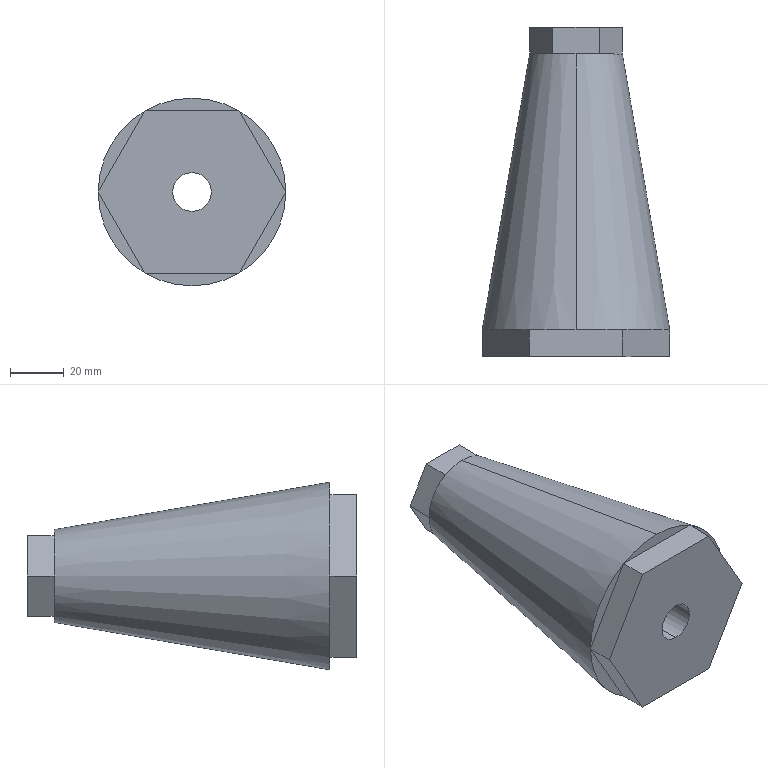Part | SolidWorks | features Extrusion 1, HoleWzd 1, ICE 1, Revolution 1 | 1 solid | 30 faces | box 70 x 123 x 70 mm | volume 249186 mm3 | plane 26 | cylinder 2 | cone 2 | commonest cylinder face diameters 14.5 x2
STEP:
#1=CARTESIAN_POINT('',(0.,-113.,-7.25));
#2=VERTEX_POINT('',#1);
#3=CARTESIAN_POINT('',(0.,-113.,7.25));
#4=VERTEX_POINT('',#3);
#5=CARTESIAN_POINT('',(0.,-113.,0.));
#6=DIRECTION('',(0.,1.,0.));
#7=DIRECTION('',(0.,0.,1.));
#8=AXIS2_PLACEMENT_3D('',#5,#6,#7);
#9=CIRCLE('',#8,7.25);
#10=EDGE_CURVE('',#2,#4,#9,.T.);
#11=ORIENTED_EDGE('',*,*,#10,.F.);
#12=CARTESIAN_POINT('',(0.,10.,-7.25));
#13=VERTEX_POINT('',#12);
#14=CARTESIAN_POINT('',(0.,10.,-7.25));
#15=DIRECTION('',(0.,1.,0.));
#16=VECTOR('',#15,1000.);
#17=LINE('',#14,#16);
#18=EDGE_CURVE('',#2,#13,#17,.T.);
#19=ORIENTED_EDGE('',*,*,#18,.T.);
#20=CARTESIAN_POINT('',(0.,10.,7.25));
#21=VERTEX_POINT('',#20);
#22=CARTESIAN_POINT('',(0.,10.,0.));
#23=DIRECTION('',(0.,1.,0.));
#24=DIRECTION('',(0.,0.,1.));
#25=AXIS2_PLACEMENT_3D('',#22,#23,#24);
#26=CIRCLE('',#25,7.25);
#27=EDGE_CURVE('',#13,#21,#26,.T.);
#28=ORIENTED_EDGE('',*,*,#27,.T.);
#29=CARTESIAN_POINT('',(0.,10.,7.25));
#30=DIRECTION('',(0.,1.,0.));
#31=VECTOR('',#30,1000.);
#32=LINE('',#29,#31);
#33=EDGE_CURVE('',#4,#21,#32,.T.);
#34=ORIENTED_EDGE('',*,*,#33,.F.);
#35=EDGE_LOOP('',(#11,#19,#28,#34));
#36=FACE_OUTER_BOUND('',#35,.T.);
#37=CARTESIAN_POINT('',(0.,10.,0.));
#38=DIRECTION('',(0.,1.,0.));
#39=DIRECTION('',(0.,0.,1.));
#40=AXIS2_PLACEMENT_3D('',#37,#38,#39);
#41=CYLINDRICAL_SURFACE('',#40,7.25);
#42=ADVANCED_FACE('',(#36),#41,.F.);
#43=CARTESIAN_POINT('',(8.66,0.,15.));
#44=VERTEX_POINT('',#43);
#45=CARTESIAN_POINT('',(0.,0.,17.321));
#46=VERTEX_POINT('',#45);
#47=CARTESIAN_POINT('',(0.,0.,0.));
#48=DIRECTION('',(0.,-1.,0.));
#49=DIRECTION('',(0.,0.,-1.));
#50=AXIS2_PLACEMENT_3D('',#47,#48,#49);
#51=CIRCLE('',#50,17.321);
#52=EDGE_CURVE('',#44,#46,#51,.T.);
#53=ORIENTED_EDGE('',*,*,#52,.T.);
#54=CARTESIAN_POINT('',(0.,-103.,35.));
#55=VERTEX_POINT('',#54);
#56=CARTESIAN_POINT('',(0.,-103.,35.));
#57=DIRECTION('',(0.,-0.9856,0.1692));
#58=VECTOR('',#57,1000.);
#59=LINE('',#56,#58);
#60=EDGE_CURVE('',#46,#55,#59,.T.);
#61=ORIENTED_EDGE('',*,*,#60,.T.);
#62=CARTESIAN_POINT('',(17.5,-103.,30.311));
#63=VERTEX_POINT('',#62);
#64=CARTESIAN_POINT('',(0.,-103.,0.));
#65=DIRECTION('',(0.,-1.,0.));
#66=DIRECTION('',(0.,0.,-1.));
#67=AXIS2_PLACEMENT_3D('',#64,#65,#66);
#68=CIRCLE('',#67,35.);
#69=EDGE_CURVE('',#63,#55,#68,.T.);
#70=ORIENTED_EDGE('',*,*,#69,.F.);
#71=CARTESIAN_POINT('',(35.,-103.,0.));
#72=VERTEX_POINT('',#71);
#73=CARTESIAN_POINT('',(0.,-103.,0.));
#74=DIRECTION('',(0.,-1.,0.));
#75=DIRECTION('',(0.,0.,-1.));
#76=AXIS2_PLACEMENT_3D('',#73,#74,#75);
#77=CIRCLE('',#76,35.);
#78=EDGE_CURVE('',#72,#63,#77,.T.);
#79=ORIENTED_EDGE('',*,*,#78,.F.);
#80=CARTESIAN_POINT('',(17.5,-103.,-30.311));
#81=VERTEX_POINT('',#80);
#82=CARTESIAN_POINT('',(0.,-103.,0.));
#83=DIRECTION('',(0.,-1.,0.));
#84=DIRECTION('',(0.,0.,-1.));
#85=AXIS2_PLACEMENT_3D('',#82,#83,#84);
#86=CIRCLE('',#85,35.);
#87=EDGE_CURVE('',#81,#72,#86,.T.);
#88=ORIENTED_EDGE('',*,*,#87,.F.);
#89=CARTESIAN_POINT('',(0.,-103.,-35.));
#90=VERTEX_POINT('',#89);
#91=CARTESIAN_POINT('',(0.,-103.,0.));
#92=DIRECTION('',(0.,-1.,0.));
#93=DIRECTION('',(0.,0.,-1.));
#94=AXIS2_PLACEMENT_3D('',#91,#92,#93);
#95=CIRCLE('',#94,35.);
#96=EDGE_CURVE('',#90,#81,#95,.T.);
#97=ORIENTED_EDGE('',*,*,#96,.F.);
#98=CARTESIAN_POINT('',(0.,0.,-17.321));
#99=VERTEX_POINT('',#98);
#100=CARTESIAN_POINT('',(0.,-103.,-35.));
#101=DIRECTION('',(0.,-0.9856,-0.1692));
#102=VECTOR('',#101,1000.);
#103=LINE('',#100,#102);
#104=EDGE_CURVE('',#99,#90,#103,.T.);
#105=ORIENTED_EDGE('',*,*,#104,.F.);
#106=CARTESIAN_POINT('',(8.66,0.,-15.));
#107=VERTEX_POINT('',#106);
#108=CARTESIAN_POINT('',(0.,0.,0.));
#109=DIRECTION('',(0.,-1.,0.));
#110=DIRECTION('',(0.,0.,-1.));
#111=AXIS2_PLACEMENT_3D('',#108,#109,#110);
#112=CIRCLE('',#111,17.321);
#113=EDGE_CURVE('',#99,#107,#112,.T.);
#114=ORIENTED_EDGE('',*,*,#113,.T.);
#115=CARTESIAN_POINT('',(17.321,0.,0.));
#116=VERTEX_POINT('',#115);
#117=CARTESIAN_POINT('',(0.,0.,0.));
#118=DIRECTION('',(0.,-1.,0.));
#119=DIRECTION('',(0.,0.,-1.));
#120=AXIS2_PLACEMENT_3D('',#117,#118,#119);
#121=CIRCLE('',#120,17.321);
#122=EDGE_CURVE('',#107,#116,#121,.T.);
#123=ORIENTED_EDGE('',*,*,#122,.T.);
#124=CARTESIAN_POINT('',(0.,0.,0.));
#125=DIRECTION('',(0.,-1.,0.));
#126=DIRECTION('',(0.,0.,-1.));
#127=AXIS2_PLACEMENT_3D('',#124,#125,#126);
#128=CIRCLE('',#127,17.321);
#129=EDGE_CURVE('',#116,#44,#128,.T.);
#130=ORIENTED_EDGE('',*,*,#129,.T.);
#131=EDGE_LOOP('',(#53,#61,#70,#79,#88,#97,#105,#114,#123,#130));
#132=FACE_OUTER_BOUND('',#131,.T.);
#133=CARTESIAN_POINT('',(0.,-103.,0.));
#134=DIRECTION('',(0.,-1.,0.));
#135=DIRECTION('',(0.,0.,-1.));
#136=AXIS2_PLACEMENT_3D('',#133,#134,#135);
#137=CONICAL_SURFACE('',#136,35.,0.17);
#138=ADVANCED_FACE('',(#132),#137,.T.);
#139=CARTESIAN_POINT('',(35.,-103.,0.));
#140=DIRECTION('',(-0.5,0.,0.866));
#141=VECTOR('',#140,1000.);
#142=LINE('',#139,#141);
#143=EDGE_CURVE('',#72,#63,#142,.T.);
#144=ORIENTED_EDGE('',*,*,#143,.F.);
#145=ORIENTED_EDGE('',*,*,#78,.T.);
#146=EDGE_LOOP('',(#144,#145));
#147=FACE_OUTER_BOUND('',#146,.T.);
#148=CARTESIAN_POINT('',(35.,-103.,0.));
#149=DIRECTION('',(0.,-1.,0.));
#150=DIRECTION('',(0.,0.,-1.));
#151=AXIS2_PLACEMENT_3D('',#148,#149,#150);
#152=PLANE('',#151);
#153=ADVANCED_FACE('',(#147),#152,.T.);
#154=CARTESIAN_POINT('',(17.5,-103.,-30.311));
#155=DIRECTION('',(0.5,0.,0.866));
#156=VECTOR('',#155,1000.);
#157=LINE('',#154,#156);
#158=EDGE_CURVE('',#81,#72,#157,.T.);
#159=ORIENTED_EDGE('',*,*,#158,.F.);
#160=ORIENTED_EDGE('',*,*,#87,.T.);
#161=EDGE_LOOP('',(#159,#160));
#162=FACE_OUTER_BOUND('',#161,.T.);
#163=CARTESIAN_POINT('',(35.,-103.,0.));
#164=DIRECTION('',(0.,-1.,0.));
#165=DIRECTION('',(0.,0.,-1.));
#166=AXIS2_PLACEMENT_3D('',#163,#164,#165);
#167=PLANE('',#166);
#168=ADVANCED_FACE('',(#162),#167,.T.);
#169=CARTESIAN_POINT('',(-17.5,-103.,-30.311));
#170=VERTEX_POINT('',#169);
#171=CARTESIAN_POINT('',(-17.5,-103.,-30.311));
#172=DIRECTION('',(1.,0.,0.));
#173=VECTOR('',#172,1000.);
#174=LINE('',#171,#173);
#175=EDGE_CURVE('',#170,#81,#174,.T.);
#176=ORIENTED_EDGE('',*,*,#175,.F.);
#177=CARTESIAN_POINT('',(0.,-103.,0.));
#178=DIRECTION('',(0.,-1.,0.));
#179=DIRECTION('',(0.,0.,-1.));
#180=AXIS2_PLACEMENT_3D('',#177,#178,#179);
#181=CIRCLE('',#180,35.);
#182=EDGE_CURVE('',#170,#90,#181,.T.);
#183=ORIENTED_EDGE('',*,*,#182,.T.);
#184=ORIENTED_EDGE('',*,*,#96,.T.);
#185=EDGE_LOOP('',(#176,#183,#184));
#186=FACE_OUTER_BOUND('',#185,.T.);
#187=CARTESIAN_POINT('',(35.,-103.,0.));
#188=DIRECTION('',(0.,-1.,0.));
#189=DIRECTION('',(0.,0.,-1.));
#190=AXIS2_PLACEMENT_3D('',#187,#188,#189);
#191=PLANE('',#190);
#192=ADVANCED_FACE('',(#186),#191,.T.);
#193=CARTESIAN_POINT('',(-35.,-103.,0.));
#194=VERTEX_POINT('',#193);
#195=CARTESIAN_POINT('',(-35.,-103.,0.));
#196=DIRECTION('',(0.5,0.,-0.866));
#197=VECTOR('',#196,1000.);
#198=LINE('',#195,#197);
#199=EDGE_CURVE('',#194,#170,#198,.T.);
#200=ORIENTED_EDGE('',*,*,#199,.F.);
#201=CARTESIAN_POINT('',(0.,-103.,0.));
#202=DIRECTION('',(0.,-1.,0.));
#203=DIRECTION('',(0.,0.,-1.));
#204=AXIS2_PLACEMENT_3D('',#201,#202,#203);
#205=CIRCLE('',#204,35.);
#206=EDGE_CURVE('',#194,#170,#205,.T.);
#207=ORIENTED_EDGE('',*,*,#206,.T.);
#208=EDGE_LOOP('',(#200,#207));
#209=FACE_OUTER_BOUND('',#208,.T.);
#210=CARTESIAN_POINT('',(35.,-103.,0.));
#211=DIRECTION('',(0.,-1.,0.));
#212=DIRECTION('',(0.,0.,-1.));
#213=AXIS2_PLACEMENT_3D('',#210,#211,#212);
#214=PLANE('',#213);
#215=ADVANCED_FACE('',(#209),#214,.T.);
#216=CARTESIAN_POINT('',(-17.5,-103.,30.311));
#217=VERTEX_POINT('',#216);
#218=CARTESIAN_POINT('',(-17.5,-103.,30.311));
#219=DIRECTION('',(-0.5,0.,-0.866));
#220=VECTOR('',#219,1000.);
#221=LINE('',#218,#220);
#222=EDGE_CURVE('',#217,#194,#221,.T.);
#223=ORIENTED_EDGE('',*,*,#222,.F.);
#224=CARTESIAN_POINT('',(0.,-103.,0.));
#225=DIRECTION('',(0.,-1.,0.));
#226=DIRECTION('',(0.,0.,-1.));
#227=AXIS2_PLACEMENT_3D('',#224,#225,#226);
#228=CIRCLE('',#227,35.);
#229=EDGE_CURVE('',#217,#194,#228,.T.);
#230=ORIENTED_EDGE('',*,*,#229,.T.);
#231=EDGE_LOOP('',(#223,#230));
#232=FACE_OUTER_BOUND('',#231,.T.);
#233=CARTESIAN_POINT('',(35.,-103.,0.));
#234=DIRECTION('',(0.,-1.,0.));
#235=DIRECTION('',(0.,0.,-1.));
#236=AXIS2_PLACEMENT_3D('',#233,#234,#235);
#237=PLANE('',#236);
#238=ADVANCED_FACE('',(#232),#237,.T.);
#239=CARTESIAN_POINT('',(-8.66,0.,15.));
#240=VERTEX_POINT('',#239);
#241=CARTESIAN_POINT('',(-8.66,0.,15.));
#242=DIRECTION('',(1.,0.,0.));
#243=VECTOR('',#242,1000.);
#244=LINE('',#241,#243);
#245=EDGE_CURVE('',#240,#44,#244,.T.);
#246=ORIENTED_EDGE('',*,*,#245,.T.);
#247=CARTESIAN_POINT('',(8.66,10.,15.));
#248=VERTEX_POINT('',#247);
#249=CARTESIAN_POINT('',(8.66,10.,15.));
#250=DIRECTION('',(0.,-1.,0.));
#251=VECTOR('',#250,1000.);
#252=LINE('',#249,#251);
#253=EDGE_CURVE('',#248,#44,#252,.T.);
#254=ORIENTED_EDGE('',*,*,#253,.F.);
#255=CARTESIAN_POINT('',(-8.66,10.,15.));
#256=VERTEX_POINT('',#255);
#257=CARTESIAN_POINT('',(-8.66,10.,15.));
#258=DIRECTION('',(1.,0.,0.));
#259=VECTOR('',#258,1000.);
#260=LINE('',#257,#259);
#261=EDGE_CURVE('',#256,#248,#260,.T.);
#262=ORIENTED_EDGE('',*,*,#261,.F.);
#263=CARTESIAN_POINT('',(-8.66,10.,15.));
#264=DIRECTION('',(0.,-1.,0.));
#265=VECTOR('',#264,1000.);
#266=LINE('',#263,#265);
#267=EDGE_CURVE('',#256,#240,#266,.T.);
#268=ORIENTED_EDGE('',*,*,#267,.T.);
#269=EDGE_LOOP('',(#246,#254,#262,#268));
#270=FACE_OUTER_BOUND('',#269,.T.);
#271=CARTESIAN_POINT('',(-8.66,10.,15.));
#272=DIRECTION('',(0.,0.,-1.));
#273=DIRECTION('',(-1.,0.,0.));
#274=AXIS2_PLACEMENT_3D('',#271,#272,#273);
#275=PLANE('',#274);
#276=ADVANCED_FACE('',(#270),#275,.F.);
#277=CARTESIAN_POINT('',(8.66,0.,15.));
#278=DIRECTION('',(0.5,0.,-0.866));
#279=VECTOR('',#278,1000.);
#280=LINE('',#277,#279);
#281=EDGE_CURVE('',#44,#116,#280,.T.);
#282=ORIENTED_EDGE('',*,*,#281,.T.);
#283=CARTESIAN_POINT('',(17.321,10.,0.));
#284=VERTEX_POINT('',#283);
#285=CARTESIAN_POINT('',(17.321,10.,0.));
#286=DIRECTION('',(0.,-1.,0.));
#287=VECTOR('',#286,1000.);
#288=LINE('',#285,#287);
#289=EDGE_CURVE('',#284,#116,#288,.T.);
#290=ORIENTED_EDGE('',*,*,#289,.F.);
#291=CARTESIAN_POINT('',(8.66,10.,15.));
#292=DIRECTION('',(0.5,0.,-0.866));
#293=VECTOR('',#292,1000.);
#294=LINE('',#291,#293);
#295=EDGE_CURVE('',#248,#284,#294,.T.);
#296=ORIENTED_EDGE('',*,*,#295,.F.);
#297=ORIENTED_EDGE('',*,*,#253,.T.);
#298=EDGE_LOOP('',(#282,#290,#296,#297));
#299=FACE_OUTER_BOUND('',#298,.T.);
#300=CARTESIAN_POINT('',(8.66,10.,15.));
#301=DIRECTION('',(-0.866,0.,-0.5));
#302=DIRECTION('',(-0.5,0.,0.866));
#303=AXIS2_PLACEMENT_3D('',#300,#301,#302);
#304=PLANE('',#303);
#305=ADVANCED_FACE('',(#299),#304,.F.);
#306=CARTESIAN_POINT('',(17.321,0.,0.));
#307=DIRECTION('',(-0.5,0.,-0.866));
#308=VECTOR('',#307,1000.);
#309=LINE('',#306,#308);
#310=EDGE_CURVE('',#116,#107,#309,.T.);
#311=ORIENTED_EDGE('',*,*,#310,.T.);
#312=CARTESIAN_POINT('',(8.66,10.,-15.));
#313=VERTEX_POINT('',#312);
#314=CARTESIAN_POINT('',(8.66,10.,-15.));
#315=DIRECTION('',(0.,-1.,0.));
#316=VECTOR('',#315,1000.);
#317=LINE('',#314,#316);
#318=EDGE_CURVE('',#313,#107,#317,.T.);
#319=ORIENTED_EDGE('',*,*,#318,.F.);
#320=CARTESIAN_POINT('',(17.321,10.,0.));
#321=DIRECTION('',(-0.5,0.,-0.866));
#322=VECTOR('',#321,1000.);
#323=LINE('',#320,#322);
#324=EDGE_CURVE('',#284,#313,#323,.T.);
#325=ORIENTED_EDGE('',*,*,#324,.F.);
#326=ORIENTED_EDGE('',*,*,#289,.T.);
#327=EDGE_LOOP('',(#311,#319,#325,#326));
#328=FACE_OUTER_BOUND('',#327,.T.);
#329=CARTESIAN_POINT('',(17.321,10.,0.));
#330=DIRECTION('',(-0.866,0.,0.5));
#331=DIRECTION('',(0.5,0.,0.866));
#332=AXIS2_PLACEMENT_3D('',#329,#330,#331);
#333=PLANE('',#332);
#334=ADVANCED_FACE('',(#328),#333,.F.);
#335=CARTESIAN_POINT('',(-8.66,0.,-15.));
#336=VERTEX_POINT('',#335);
#337=CARTESIAN_POINT('',(8.66,0.,-15.));
#338=DIRECTION('',(-1.,0.,0.));
#339=VECTOR('',#338,1000.);
#340=LINE('',#337,#339);
#341=EDGE_CURVE('',#107,#336,#340,.T.);
#342=ORIENTED_EDGE('',*,*,#341,.T.);
#343=CARTESIAN_POINT('',(-8.66,10.,-15.));
#344=VERTEX_POINT('',#343);
#345=CARTESIAN_POINT('',(-8.66,10.,-15.));
#346=DIRECTION('',(0.,-1.,0.));
#347=VECTOR('',#346,1000.);
#348=LINE('',#345,#347);
#349=EDGE_CURVE('',#344,#336,#348,.T.);
#350=ORIENTED_EDGE('',*,*,#349,.F.);
#351=CARTESIAN_POINT('',(8.66,10.,-15.));
#352=DIRECTION('',(-1.,0.,0.));
#353=VECTOR('',#352,1000.);
#354=LINE('',#351,#353);
#355=EDGE_CURVE('',#313,#344,#354,.T.);
#356=ORIENTED_EDGE('',*,*,#355,.F.);
#357=ORIENTED_EDGE('',*,*,#318,.T.);
#358=EDGE_LOOP('',(#342,#350,#356,#357));
#359=FACE_OUTER_BOUND('',#358,.T.);
#360=CARTESIAN_POINT('',(8.66,10.,-15.));
#361=DIRECTION('',(0.,0.,1.));
#362=DIRECTION('',(1.,0.,0.));
#363=AXIS2_PLACEMENT_3D('',#360,#361,#362);
#364=PLANE('',#363);
#365=ADVANCED_FACE('',(#359),#364,.F.);
#366=CARTESIAN_POINT('',(-17.321,0.,0.));
#367=VERTEX_POINT('',#366);
#368=CARTESIAN_POINT('',(-8.66,0.,-15.));
#369=DIRECTION('',(-0.5,0.,0.866));
#370=VECTOR('',#369,1000.);
#371=LINE('',#368,#370);
#372=EDGE_CURVE('',#336,#367,#371,.T.);
#373=ORIENTED_EDGE('',*,*,#372,.T.);
#374=CARTESIAN_POINT('',(-17.321,10.,0.));
#375=VERTEX_POINT('',#374);
#376=CARTESIAN_POINT('',(-17.321,10.,0.));
#377=DIRECTION('',(0.,-1.,0.));
#378=VECTOR('',#377,1000.);
#379=LINE('',#376,#378);
#380=EDGE_CURVE('',#375,#367,#379,.T.);
#381=ORIENTED_EDGE('',*,*,#380,.F.);
#382=CARTESIAN_POINT('',(-8.66,10.,-15.));
#383=DIRECTION('',(-0.5,0.,0.866));
#384=VECTOR('',#383,1000.);
#385=LINE('',#382,#384);
#386=EDGE_CURVE('',#344,#375,#385,.T.);
#387=ORIENTED_EDGE('',*,*,#386,.F.);
#388=ORIENTED_EDGE('',*,*,#349,.T.);
#389=EDGE_LOOP('',(#373,#381,#387,#388));
#390=FACE_OUTER_BOUND('',#389,.T.);
#391=CARTESIAN_POINT('',(-8.66,10.,-15.));
#392=DIRECTION('',(0.866,0.,0.5));
#393=DIRECTION('',(0.5,0.,-0.866));
#394=AXIS2_PLACEMENT_3D('',#391,#392,#393);
#395=PLANE('',#394);
#396=ADVANCED_FACE('',(#390),#395,.F.);
#397=CARTESIAN_POINT('',(-17.321,0.,0.));
#398=DIRECTION('',(0.5,0.,0.866));
#399=VECTOR('',#398,1000.);
#400=LINE('',#397,#399);
#401=EDGE_CURVE('',#367,#240,#400,.T.);
#402=ORIENTED_EDGE('',*,*,#401,.T.);
#403=ORIENTED_EDGE('',*,*,#267,.F.);
#404=CARTESIAN_POINT('',(-17.321,10.,0.));
#405=DIRECTION('',(0.5,0.,0.866));
#406=VECTOR('',#405,1000.);
#407=LINE('',#404,#406);
#408=EDGE_CURVE('',#375,#256,#407,.T.);
#409=ORIENTED_EDGE('',*,*,#408,.F.);
#410=ORIENTED_EDGE('',*,*,#380,.T.);
#411=EDGE_LOOP('',(#402,#403,#409,#410));
#412=FACE_OUTER_BOUND('',#411,.T.);
#413=CARTESIAN_POINT('',(-17.321,10.,0.));
#414=DIRECTION('',(0.866,0.,-0.5));
#415=DIRECTION('',(-0.5,0.,-0.866));
#416=AXIS2_PLACEMENT_3D('',#413,#414,#415);
#417=PLANE('',#416);
#418=ADVANCED_FACE('',(#412),#417,.F.);
#419=CARTESIAN_POINT('',(0.,10.,0.));
#420=DIRECTION('',(0.,1.,0.));
#421=DIRECTION('',(0.,0.,1.));
#422=AXIS2_PLACEMENT_3D('',#419,#420,#421);
#423=CIRCLE('',#422,7.25);
#424=EDGE_CURVE('',#21,#13,#423,.T.);
#425=ORIENTED_EDGE('',*,*,#424,.F.);
#426=ORIENTED_EDGE('',*,*,#27,.F.);
#427=EDGE_LOOP('',(#425,#426));
#428=FACE_BOUND('',#427,.T.);
#429=ORIENTED_EDGE('',*,*,#261,.T.);
#430=ORIENTED_EDGE('',*,*,#295,.T.);
#431=ORIENTED_EDGE('',*,*,#324,.T.);
#432=ORIENTED_EDGE('',*,*,#355,.T.);
#433=ORIENTED_EDGE('',*,*,#386,.T.);
#434=ORIENTED_EDGE('',*,*,#408,.T.);
#435=EDGE_LOOP('',(#429,#430,#431,#432,#433,#434));
#436=FACE_OUTER_BOUND('',#435,.T.);
#437=CARTESIAN_POINT('',(0.,10.,0.));
#438=DIRECTION('',(0.,1.,0.));
#439=DIRECTION('',(0.,0.,1.));
#440=AXIS2_PLACEMENT_3D('',#437,#438,#439);
#441=PLANE('',#440);
#442=ADVANCED_FACE('',(#428,#436),#441,.T.);
#443=ORIENTED_EDGE('',*,*,#245,.F.);
#444=CARTESIAN_POINT('',(0.,0.,0.));
#445=DIRECTION('',(0.,-1.,0.));
#446=DIRECTION('',(0.,0.,-1.));
#447=AXIS2_PLACEMENT_3D('',#444,#445,#446);
#448=CIRCLE('',#447,17.321);
#449=EDGE_CURVE('',#46,#240,#448,.T.);
#450=ORIENTED_EDGE('',*,*,#449,.F.);
#451=ORIENTED_EDGE('',*,*,#52,.F.);
#452=EDGE_LOOP('',(#443,#450,#451));
#453=FACE_OUTER_BOUND('',#452,.T.);
#454=CARTESIAN_POINT('',(0.,0.,0.));
#455=DIRECTION('',(0.,1.,0.));
#456=DIRECTION('',(0.,0.,1.));
#457=AXIS2_PLACEMENT_3D('',#454,#455,#456);
#458=PLANE('',#457);
#459=ADVANCED_FACE('',(#453),#458,.T.);
#460=ORIENTED_EDGE('',*,*,#401,.F.);
#461=CARTESIAN_POINT('',(0.,0.,0.));
#462=DIRECTION('',(0.,-1.,0.));
#463=DIRECTION('',(0.,0.,-1.));
#464=AXIS2_PLACEMENT_3D('',#461,#462,#463);
#465=CIRCLE('',#464,17.321);
#466=EDGE_CURVE('',#240,#367,#465,.T.);
#467=ORIENTED_EDGE('',*,*,#466,.F.);
#468=EDGE_LOOP('',(#460,#467));
#469=FACE_OUTER_BOUND('',#468,.T.);
#470=CARTESIAN_POINT('',(0.,0.,0.));
#471=DIRECTION('',(0.,1.,0.));
#472=DIRECTION('',(0.,0.,1.));
#473=AXIS2_PLACEMENT_3D('',#470,#471,#472);
#474=PLANE('',#473);
#475=ADVANCED_FACE('',(#469),#474,.T.);
#476=ORIENTED_EDGE('',*,*,#372,.F.);
#477=CARTESIAN_POINT('',(0.,0.,0.));
#478=DIRECTION('',(0.,-1.,0.));
#479=DIRECTION('',(0.,0.,-1.));
#480=AXIS2_PLACEMENT_3D('',#477,#478,#479);
#481=CIRCLE('',#480,17.321);
#482=EDGE_CURVE('',#367,#336,#481,.T.);
#483=ORIENTED_EDGE('',*,*,#482,.F.);
#484=EDGE_LOOP('',(#476,#483));
#485=FACE_OUTER_BOUND('',#484,.T.);
#486=CARTESIAN_POINT('',(0.,0.,0.));
#487=DIRECTION('',(0.,1.,0.));
#488=DIRECTION('',(0.,0.,1.));
#489=AXIS2_PLACEMENT_3D('',#486,#487,#488);
#490=PLANE('',#489);
#491=ADVANCED_FACE('',(#485),#490,.T.);
#492=ORIENTED_EDGE('',*,*,#341,.F.);
#493=ORIENTED_EDGE('',*,*,#113,.F.);
#494=CARTESIAN_POINT('',(0.,0.,0.));
#495=DIRECTION('',(0.,-1.,0.));
#496=DIRECTION('',(0.,0.,-1.));
#497=AXIS2_PLACEMENT_3D('',#494,#495,#496);
#498=CIRCLE('',#497,17.321);
#499=EDGE_CURVE('',#336,#99,#498,.T.);
#500=ORIENTED_EDGE('',*,*,#499,.F.);
#501=EDGE_LOOP('',(#492,#493,#500));
#502=FACE_OUTER_BOUND('',#501,.T.);
#503=CARTESIAN_POINT('',(0.,0.,0.));
#504=DIRECTION('',(0.,1.,0.));
#505=DIRECTION('',(0.,0.,1.));
#506=AXIS2_PLACEMENT_3D('',#503,#504,#505);
#507=PLANE('',#506);
#508=ADVANCED_FACE('',(#502),#507,.T.);
#509=ORIENTED_EDGE('',*,*,#310,.F.);
#510=ORIENTED_EDGE('',*,*,#122,.F.);
#511=EDGE_LOOP('',(#509,#510));
#512=FACE_OUTER_BOUND('',#511,.T.);
#513=CARTESIAN_POINT('',(0.,0.,0.));
#514=DIRECTION('',(0.,1.,0.));
#515=DIRECTION('',(0.,0.,1.));
#516=AXIS2_PLACEMENT_3D('',#513,#514,#515);
#517=PLANE('',#516);
#518=ADVANCED_FACE('',(#512),#517,.T.);
#519=ORIENTED_EDGE('',*,*,#281,.F.);
#520=ORIENTED_EDGE('',*,*,#129,.F.);
#521=EDGE_LOOP('',(#519,#520));
#522=FACE_OUTER_BOUND('',#521,.T.);
#523=CARTESIAN_POINT('',(0.,0.,0.));
#524=DIRECTION('',(0.,1.,0.));
#525=DIRECTION('',(0.,0.,1.));
#526=AXIS2_PLACEMENT_3D('',#523,#524,#525);
#527=PLANE('',#526);
#528=ADVANCED_FACE('',(#522),#527,.T.);
#529=ORIENTED_EDGE('',*,*,#60,.F.);
#530=ORIENTED_EDGE('',*,*,#449,.T.);
#531=ORIENTED_EDGE('',*,*,#466,.T.);
#532=ORIENTED_EDGE('',*,*,#482,.T.);
#533=ORIENTED_EDGE('',*,*,#499,.T.);
#534=ORIENTED_EDGE('',*,*,#104,.T.);
#535=ORIENTED_EDGE('',*,*,#182,.F.);
#536=ORIENTED_EDGE('',*,*,#206,.F.);
#537=ORIENTED_EDGE('',*,*,#229,.F.);
#538=CARTESIAN_POINT('',(0.,-103.,0.));
#539=DIRECTION('',(0.,-1.,0.));
#540=DIRECTION('',(0.,0.,-1.));
#541=AXIS2_PLACEMENT_3D('',#538,#539,#540);
#542=CIRCLE('',#541,35.);
#543=EDGE_CURVE('',#55,#217,#542,.T.);
#544=ORIENTED_EDGE('',*,*,#543,.F.);
#545=EDGE_LOOP('',(#529,#530,#531,#532,#533,#534,#535,#536,#537,#544));
#546=FACE_OUTER_BOUND('',#545,.T.);
#547=CARTESIAN_POINT('',(0.,-103.,0.));
#548=DIRECTION('',(0.,-1.,0.));
#549=DIRECTION('',(0.,0.,-1.));
#550=AXIS2_PLACEMENT_3D('',#547,#548,#549);
#551=CONICAL_SURFACE('',#550,35.,0.17);
#552=ADVANCED_FACE('',(#546),#551,.T.);
#553=CARTESIAN_POINT('',(17.5,-103.,30.311));
#554=DIRECTION('',(-1.,0.,0.));
#555=VECTOR('',#554,1000.);
#556=LINE('',#553,#555);
#557=EDGE_CURVE('',#63,#217,#556,.T.);
#558=ORIENTED_EDGE('',*,*,#557,.F.);
#559=ORIENTED_EDGE('',*,*,#69,.T.);
#560=ORIENTED_EDGE('',*,*,#543,.T.);
#561=EDGE_LOOP('',(#558,#559,#560));
#562=FACE_OUTER_BOUND('',#561,.T.);
#563=CARTESIAN_POINT('',(35.,-103.,0.));
#564=DIRECTION('',(0.,-1.,0.));
#565=DIRECTION('',(0.,0.,-1.));
#566=AXIS2_PLACEMENT_3D('',#563,#564,#565);
#567=PLANE('',#566);
#568=ADVANCED_FACE('',(#562),#567,.T.);
#569=ORIENTED_EDGE('',*,*,#143,.T.);
#570=CARTESIAN_POINT('',(17.5,-113.,30.311));
#571=VERTEX_POINT('',#570);
#572=CARTESIAN_POINT('',(17.5,-113.,30.311));
#573=DIRECTION('',(0.,1.,0.));
#574=VECTOR('',#573,1000.);
#575=LINE('',#572,#574);
#576=EDGE_CURVE('',#571,#63,#575,.T.);
#577=ORIENTED_EDGE('',*,*,#576,.F.);
#578=CARTESIAN_POINT('',(35.,-113.,0.));
#579=VERTEX_POINT('',#578);
#580=CARTESIAN_POINT('',(35.,-113.,0.));
#581=DIRECTION('',(-0.5,0.,0.866));
#582=VECTOR('',#581,1000.);
#583=LINE('',#580,#582);
#584=EDGE_CURVE('',#579,#571,#583,.T.);
#585=ORIENTED_EDGE('',*,*,#584,.F.);
#586=CARTESIAN_POINT('',(35.,-113.,0.));
#587=DIRECTION('',(0.,1.,0.));
#588=VECTOR('',#587,1000.);
#589=LINE('',#586,#588);
#590=EDGE_CURVE('',#579,#72,#589,.T.);
#591=ORIENTED_EDGE('',*,*,#590,.T.);
#592=EDGE_LOOP('',(#569,#577,#585,#591));
#593=FACE_OUTER_BOUND('',#592,.T.);
#594=CARTESIAN_POINT('',(35.,-113.,0.));
#595=DIRECTION('',(-0.866,0.,-0.5));
#596=DIRECTION('',(-0.5,0.,0.866));
#597=AXIS2_PLACEMENT_3D('',#594,#595,#596);
#598=PLANE('',#597);
#599=ADVANCED_FACE('',(#593),#598,.F.);
#600=ORIENTED_EDGE('',*,*,#557,.T.);
#601=CARTESIAN_POINT('',(-17.5,-113.,30.311));
#602=VERTEX_POINT('',#601);
#603=CARTESIAN_POINT('',(-17.5,-113.,30.311));
#604=DIRECTION('',(0.,1.,0.));
#605=VECTOR('',#604,1000.);
#606=LINE('',#603,#605);
#607=EDGE_CURVE('',#602,#217,#606,.T.);
#608=ORIENTED_EDGE('',*,*,#607,.F.);
#609=CARTESIAN_POINT('',(17.5,-113.,30.311));
#610=DIRECTION('',(-1.,0.,0.));
#611=VECTOR('',#610,1000.);
#612=LINE('',#609,#611);
#613=EDGE_CURVE('',#571,#602,#612,.T.);
#614=ORIENTED_EDGE('',*,*,#613,.F.);
#615=ORIENTED_EDGE('',*,*,#576,.T.);
#616=EDGE_LOOP('',(#600,#608,#614,#615));
#617=FACE_OUTER_BOUND('',#616,.T.);
#618=CARTESIAN_POINT('',(17.5,-113.,30.311));
#619=DIRECTION('',(0.,0.,-1.));
#620=DIRECTION('',(-1.,0.,0.));
#621=AXIS2_PLACEMENT_3D('',#618,#619,#620);
#622=PLANE('',#621);
#623=ADVANCED_FACE('',(#617),#622,.F.);
#624=ORIENTED_EDGE('',*,*,#222,.T.);
#625=CARTESIAN_POINT('',(-35.,-113.,0.));
#626=VERTEX_POINT('',#625);
#627=CARTESIAN_POINT('',(-35.,-113.,0.));
#628=DIRECTION('',(0.,1.,0.));
#629=VECTOR('',#628,1000.);
#630=LINE('',#627,#629);
#631=EDGE_CURVE('',#626,#194,#630,.T.);
#632=ORIENTED_EDGE('',*,*,#631,.F.);
#633=CARTESIAN_POINT('',(-17.5,-113.,30.311));
#634=DIRECTION('',(-0.5,0.,-0.866));
#635=VECTOR('',#634,1000.);
#636=LINE('',#633,#635);
#637=EDGE_CURVE('',#602,#626,#636,.T.);
#638=ORIENTED_EDGE('',*,*,#637,.F.);
#639=ORIENTED_EDGE('',*,*,#607,.T.);
#640=EDGE_LOOP('',(#624,#632,#638,#639));
#641=FACE_OUTER_BOUND('',#640,.T.);
#642=CARTESIAN_POINT('',(-17.5,-113.,30.311));
#643=DIRECTION('',(0.866,0.,-0.5));
#644=DIRECTION('',(-0.5,0.,-0.866));
#645=AXIS2_PLACEMENT_3D('',#642,#643,#644);
#646=PLANE('',#645);
#647=ADVANCED_FACE('',(#641),#646,.F.);
#648=ORIENTED_EDGE('',*,*,#199,.T.);
#649=CARTESIAN_POINT('',(-17.5,-113.,-30.311));
#650=VERTEX_POINT('',#649);
#651=CARTESIAN_POINT('',(-17.5,-113.,-30.311));
#652=DIRECTION('',(0.,1.,0.));
#653=VECTOR('',#652,1000.);
#654=LINE('',#651,#653);
#655=EDGE_CURVE('',#650,#170,#654,.T.);
#656=ORIENTED_EDGE('',*,*,#655,.F.);
#657=CARTESIAN_POINT('',(-35.,-113.,0.));
#658=DIRECTION('',(0.5,0.,-0.866));
#659=VECTOR('',#658,1000.);
#660=LINE('',#657,#659);
#661=EDGE_CURVE('',#626,#650,#660,.T.);
#662=ORIENTED_EDGE('',*,*,#661,.F.);
#663=ORIENTED_EDGE('',*,*,#631,.T.);
#664=EDGE_LOOP('',(#648,#656,#662,#663));
#665=FACE_OUTER_BOUND('',#664,.T.);
#666=CARTESIAN_POINT('',(-35.,-113.,0.));
#667=DIRECTION('',(0.866,0.,0.5));
#668=DIRECTION('',(0.5,0.,-0.866));
#669=AXIS2_PLACEMENT_3D('',#666,#667,#668);
#670=PLANE('',#669);
#671=ADVANCED_FACE('',(#665),#670,.F.);
#672=ORIENTED_EDGE('',*,*,#175,.T.);
#673=CARTESIAN_POINT('',(17.5,-113.,-30.311));
#674=VERTEX_POINT('',#673);
#675=CARTESIAN_POINT('',(17.5,-113.,-30.311));
#676=DIRECTION('',(0.,1.,0.));
#677=VECTOR('',#676,1000.);
#678=LINE('',#675,#677);
#679=EDGE_CURVE('',#674,#81,#678,.T.);
#680=ORIENTED_EDGE('',*,*,#679,.F.);
#681=CARTESIAN_POINT('',(-17.5,-113.,-30.311));
#682=DIRECTION('',(1.,0.,0.));
#683=VECTOR('',#682,1000.);
#684=LINE('',#681,#683);
#685=EDGE_CURVE('',#650,#674,#684,.T.);
#686=ORIENTED_EDGE('',*,*,#685,.F.);
#687=ORIENTED_EDGE('',*,*,#655,.T.);
#688=EDGE_LOOP('',(#672,#680,#686,#687));
#689=FACE_OUTER_BOUND('',#688,.T.);
#690=CARTESIAN_POINT('',(-17.5,-113.,-30.311));
#691=DIRECTION('',(0.,0.,1.));
#692=DIRECTION('',(1.,0.,0.));
#693=AXIS2_PLACEMENT_3D('',#690,#691,#692);
#694=PLANE('',#693);
#695=ADVANCED_FACE('',(#689),#694,.F.);
#696=ORIENTED_EDGE('',*,*,#158,.T.);
#697=ORIENTED_EDGE('',*,*,#590,.F.);
#698=CARTESIAN_POINT('',(17.5,-113.,-30.311));
#699=DIRECTION('',(0.5,0.,0.866));
#700=VECTOR('',#699,1000.);
#701=LINE('',#698,#700);
#702=EDGE_CURVE('',#674,#579,#701,.T.);
#703=ORIENTED_EDGE('',*,*,#702,.F.);
#704=ORIENTED_EDGE('',*,*,#679,.T.);
#705=EDGE_LOOP('',(#696,#697,#703,#704));
#706=FACE_OUTER_BOUND('',#705,.T.);
#707=CARTESIAN_POINT('',(17.5,-113.,-30.311));
#708=DIRECTION('',(-0.866,0.,0.5));
#709=DIRECTION('',(0.5,0.,0.866));
#710=AXIS2_PLACEMENT_3D('',#707,#708,#709);
#711=PLANE('',#710);
#712=ADVANCED_FACE('',(#706),#711,.F.);
#713=CARTESIAN_POINT('',(0.,-113.,0.));
#714=DIRECTION('',(0.,1.,0.));
#715=DIRECTION('',(0.,0.,1.));
#716=AXIS2_PLACEMENT_3D('',#713,#714,#715);
#717=CIRCLE('',#716,7.25);
#718=EDGE_CURVE('',#4,#2,#717,.T.);
#719=ORIENTED_EDGE('',*,*,#718,.T.);
#720=ORIENTED_EDGE('',*,*,#10,.T.);
#721=EDGE_LOOP('',(#719,#720));
#722=FACE_BOUND('',#721,.T.);
#723=ORIENTED_EDGE('',*,*,#584,.T.);
#724=ORIENTED_EDGE('',*,*,#613,.T.);
#725=ORIENTED_EDGE('',*,*,#637,.T.);
#726=ORIENTED_EDGE('',*,*,#661,.T.);
#727=ORIENTED_EDGE('',*,*,#685,.T.);
#728=ORIENTED_EDGE('',*,*,#702,.T.);
#729=EDGE_LOOP('',(#723,#724,#725,#726,#727,#728));
#730=FACE_OUTER_BOUND('',#729,.T.);
#731=CARTESIAN_POINT('',(0.,-113.,0.));
#732=DIRECTION('',(0.,-1.,0.));
#733=DIRECTION('',(0.,0.,-1.));
#734=AXIS2_PLACEMENT_3D('',#731,#732,#733);
#735=PLANE('',#734);
#736=ADVANCED_FACE('',(#722,#730),#735,.T.);
#737=ORIENTED_EDGE('',*,*,#18,.F.);
#738=ORIENTED_EDGE('',*,*,#718,.F.);
#739=ORIENTED_EDGE('',*,*,#33,.T.);
#740=ORIENTED_EDGE('',*,*,#424,.T.);
#741=EDGE_LOOP('',(#737,#738,#739,#740));
#742=FACE_OUTER_BOUND('',#741,.T.);
#743=CARTESIAN_POINT('',(0.,10.,0.));
#744=DIRECTION('',(0.,1.,0.));
#745=DIRECTION('',(0.,0.,1.));
#746=AXIS2_PLACEMENT_3D('',#743,#744,#745);
#747=CYLINDRICAL_SURFACE('',#746,7.25);
#748=ADVANCED_FACE('',(#742),#747,.F.);
#749=CLOSED_SHELL('',(#42,#138,#153,#168,#192,#215,#238,#276,#305,#334,#365,#396,#418,#442,#459,#475,#491,#508,#518,#528,#552,#568,#599,#623,#647,#671,#695,#712,#736,#748));
#750=MANIFOLD_SOLID_BREP('',#749);
#751=CARTESIAN_POINT('',(0.,0.,0.));
#752=DIRECTION('',(0.,0.,1.));
#753=DIRECTION('',(1.,0.,0.));
#754=AXIS2_PLACEMENT_3D('',#751,#752,#753);
#755=(LENGTH_UNIT()NAMED_UNIT(*)SI_UNIT(.MILLI.,.METRE.));
#756=UNCERTAINTY_MEASURE_WITH_UNIT(LENGTH_MEASURE(0.00001),#755,'','');
#757=(NAMED_UNIT(*)PLANE_ANGLE_UNIT()SI_UNIT($,.RADIAN.));
#758=(NAMED_UNIT(*)SI_UNIT($,.STERADIAN.)SOLID_ANGLE_UNIT());
#759=(GEOMETRIC_REPRESENTATION_CONTEXT(3)GLOBAL_UNCERTAINTY_ASSIGNED_CONTEXT((#756))GLOBAL_UNIT_ASSIGNED_CONTEXT((#755,#757,#758))REPRESENTATION_CONTEXT('',''));
#760=ADVANCED_BREP_SHAPE_REPRESENTATION('',(#750,#754),#759);